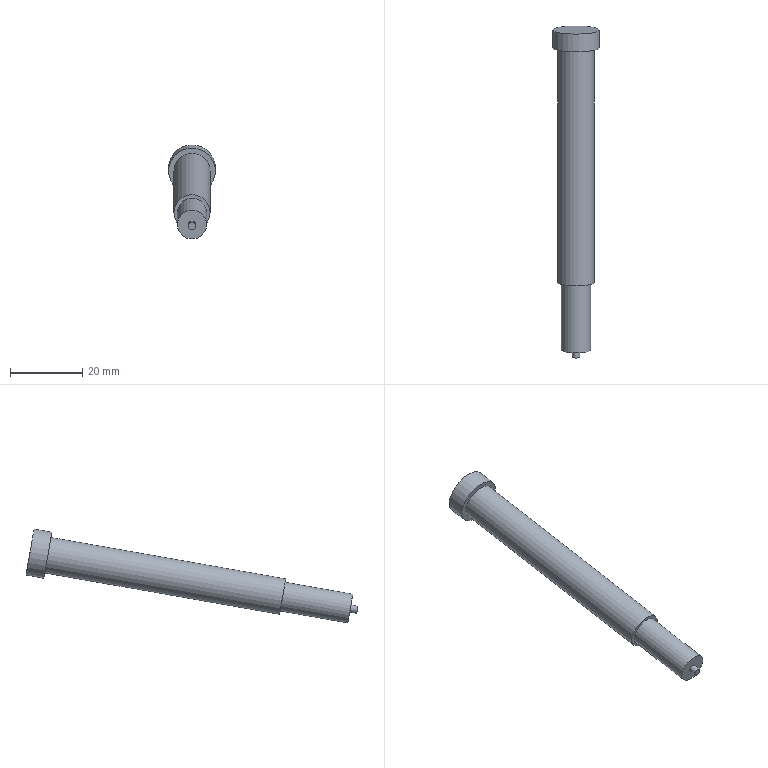Part | NX | features solid 2 | 1 solid | 9 faces | box 13 x 91.905 x 26.018 mm | volume 6833 mm3 | plane 5 | cylinder 4 | commonest cylinder face diameters 2 x1 8.1 x1 10 x1 13 x1
STEP:
#1=CARTESIAN_POINT('',(554.171,576.6,-0.1623));
#2=VERTEX_POINT('',#1);
#3=CARTESIAN_POINT('',(549.171,576.6,-0.1623));
#4=DIRECTION('',(0.,-0.9848,-0.1736));
#5=DIRECTION('',(1.,0.,0.));
#6=AXIS2_PLACEMENT_3D('',#3,#4,#5);
#7=CIRCLE('',#6,5.);
#8=EDGE_CURVE('',#2,#2,#7,.T.);
#9=ORIENTED_EDGE('',*,*,#8,.F.);
#10=EDGE_LOOP('',(#9));
#11=FACE_BOUND('',#10,.T.);
#12=CARTESIAN_POINT('',(554.171,641.597,11.298));
#13=VERTEX_POINT('',#12);
#14=CARTESIAN_POINT('',(549.171,641.597,11.298));
#15=DIRECTION('',(0.,-0.9848,-0.1736));
#16=DIRECTION('',(1.,0.,0.));
#17=AXIS2_PLACEMENT_3D('',#14,#15,#16);
#18=CIRCLE('',#17,5.);
#19=EDGE_CURVE('',#13,#13,#18,.T.);
#20=ORIENTED_EDGE('',*,*,#19,.T.);
#21=EDGE_LOOP('',(#20));
#22=FACE_BOUND('',#21,.T.);
#23=CARTESIAN_POINT('',(549.171,646.521,12.167));
#24=DIRECTION('',(0.,-0.9848,-0.1736));
#25=DIRECTION('',(-1.,0.,0.));
#26=AXIS2_PLACEMENT_3D('',#23,#24,#25);
#27=CYLINDRICAL_SURFACE('',#26,5.);
#28=ADVANCED_FACE('',(#11,#22),#27,.T.);
#29=CARTESIAN_POINT('',(553.221,576.6,-0.1623));
#30=VERTEX_POINT('',#29);
#31=CARTESIAN_POINT('',(549.171,576.6,-0.1623));
#32=DIRECTION('',(0.,-0.9848,-0.1736));
#33=DIRECTION('',(1.,0.,0.));
#34=AXIS2_PLACEMENT_3D('',#31,#32,#33);
#35=CIRCLE('',#34,4.05);
#36=EDGE_CURVE('',#30,#30,#35,.T.);
#37=ORIENTED_EDGE('',*,*,#36,.F.);
#38=EDGE_LOOP('',(#37));
#39=FACE_BOUND('',#38,.T.);
#40=ORIENTED_EDGE('',*,*,#8,.T.);
#41=EDGE_LOOP('',(#40));
#42=FACE_BOUND('',#41,.T.);
#43=CARTESIAN_POINT('',(549.171,576.6,-0.1623));
#44=DIRECTION('',(0.,0.9848,0.1736));
#45=DIRECTION('',(1.,0.,0.));
#46=AXIS2_PLACEMENT_3D('',#43,#44,#45);
#47=PLANE('',#46);
#48=ADVANCED_FACE('',(#39,#42),#47,.F.);
#49=CARTESIAN_POINT('',(555.671,641.597,11.298));
#50=VERTEX_POINT('',#49);
#51=CARTESIAN_POINT('',(549.171,641.597,11.298));
#52=DIRECTION('',(0.,-0.9848,-0.1736));
#53=DIRECTION('',(1.,0.,0.));
#54=AXIS2_PLACEMENT_3D('',#51,#52,#53);
#55=CIRCLE('',#54,6.5);
#56=EDGE_CURVE('',#50,#50,#55,.T.);
#57=ORIENTED_EDGE('',*,*,#56,.T.);
#58=EDGE_LOOP('',(#57));
#59=FACE_BOUND('',#58,.T.);
#60=ORIENTED_EDGE('',*,*,#19,.F.);
#61=EDGE_LOOP('',(#60));
#62=FACE_BOUND('',#61,.T.);
#63=CARTESIAN_POINT('',(549.171,641.597,11.298));
#64=DIRECTION('',(0.,0.9848,0.1736));
#65=DIRECTION('',(1.,0.,0.));
#66=AXIS2_PLACEMENT_3D('',#63,#64,#65);
#67=PLANE('',#66);
#68=ADVANCED_FACE('',(#59,#62),#67,.F.);
#69=ORIENTED_EDGE('',*,*,#56,.F.);
#70=EDGE_LOOP('',(#69));
#71=FACE_BOUND('',#70,.T.);
#72=CARTESIAN_POINT('',(555.671,646.521,12.167));
#73=VERTEX_POINT('',#72);
#74=CARTESIAN_POINT('',(549.171,646.521,12.167));
#75=DIRECTION('',(0.,-0.9848,-0.1736));
#76=DIRECTION('',(1.,0.,0.));
#77=AXIS2_PLACEMENT_3D('',#74,#75,#76);
#78=CIRCLE('',#77,6.5);
#79=EDGE_CURVE('',#73,#73,#78,.T.);
#80=ORIENTED_EDGE('',*,*,#79,.T.);
#81=EDGE_LOOP('',(#80));
#82=FACE_BOUND('',#81,.T.);
#83=CARTESIAN_POINT('',(549.171,641.597,11.298));
#84=DIRECTION('',(0.,0.9848,0.1736));
#85=DIRECTION('',(1.,0.,0.));
#86=AXIS2_PLACEMENT_3D('',#83,#84,#85);
#87=CYLINDRICAL_SURFACE('',#86,6.5);
#88=ADVANCED_FACE('',(#71,#82),#87,.T.);
#89=ORIENTED_EDGE('',*,*,#79,.F.);
#90=EDGE_LOOP('',(#89));
#91=FACE_BOUND('',#90,.T.);
#92=CARTESIAN_POINT('',(549.171,646.521,12.167));
#93=DIRECTION('',(0.,0.9848,0.1736));
#94=DIRECTION('',(1.,0.,0.));
#95=AXIS2_PLACEMENT_3D('',#92,#93,#94);
#96=PLANE('',#95);
#97=ADVANCED_FACE('',(#91),#96,.T.);
#98=CARTESIAN_POINT('',(553.221,557.888,-3.462));
#99=VERTEX_POINT('',#98);
#100=CARTESIAN_POINT('',(549.171,557.888,-3.462));
#101=DIRECTION('',(0.,-0.9848,-0.1736));
#102=DIRECTION('',(1.,0.,0.));
#103=AXIS2_PLACEMENT_3D('',#100,#101,#102);
#104=CIRCLE('',#103,4.05);
#105=EDGE_CURVE('',#99,#99,#104,.T.);
#106=ORIENTED_EDGE('',*,*,#105,.F.);
#107=EDGE_LOOP('',(#106));
#108=FACE_BOUND('',#107,.T.);
#109=ORIENTED_EDGE('',*,*,#36,.T.);
#110=EDGE_LOOP('',(#109));
#111=FACE_BOUND('',#110,.T.);
#112=CARTESIAN_POINT('',(549.171,557.888,-3.462));
#113=DIRECTION('',(0.,0.9848,0.1736));
#114=DIRECTION('',(1.,0.,0.));
#115=AXIS2_PLACEMENT_3D('',#112,#113,#114);
#116=CYLINDRICAL_SURFACE('',#115,4.05);
#117=ADVANCED_FACE('',(#108,#111),#116,.T.);
#118=CARTESIAN_POINT('',(550.171,557.888,-3.462));
#119=VERTEX_POINT('',#118);
#120=CARTESIAN_POINT('',(549.171,557.888,-3.462));
#121=DIRECTION('',(0.,-0.9848,-0.1736));
#122=DIRECTION('',(1.,0.,0.));
#123=AXIS2_PLACEMENT_3D('',#120,#121,#122);
#124=CIRCLE('',#123,1.);
#125=EDGE_CURVE('',#119,#119,#124,.T.);
#126=ORIENTED_EDGE('',*,*,#125,.F.);
#127=EDGE_LOOP('',(#126));
#128=FACE_BOUND('',#127,.T.);
#129=ORIENTED_EDGE('',*,*,#105,.T.);
#130=EDGE_LOOP('',(#129));
#131=FACE_BOUND('',#130,.T.);
#132=CARTESIAN_POINT('',(549.171,557.888,-3.462));
#133=DIRECTION('',(0.,0.9848,0.1736));
#134=DIRECTION('',(1.,0.,0.));
#135=AXIS2_PLACEMENT_3D('',#132,#133,#134);
#136=PLANE('',#135);
#137=ADVANCED_FACE('',(#128,#131),#136,.F.);
#138=CARTESIAN_POINT('',(550.171,555.919,-3.809));
#139=VERTEX_POINT('',#138);
#140=CARTESIAN_POINT('',(549.171,555.919,-3.809));
#141=DIRECTION('',(0.,-0.9848,-0.1736));
#142=DIRECTION('',(1.,0.,0.));
#143=AXIS2_PLACEMENT_3D('',#140,#141,#142);
#144=CIRCLE('',#143,1.);
#145=EDGE_CURVE('',#139,#139,#144,.T.);
#146=ORIENTED_EDGE('',*,*,#145,.F.);
#147=EDGE_LOOP('',(#146));
#148=FACE_BOUND('',#147,.T.);
#149=ORIENTED_EDGE('',*,*,#125,.T.);
#150=EDGE_LOOP('',(#149));
#151=FACE_BOUND('',#150,.T.);
#152=CARTESIAN_POINT('',(549.171,555.919,-3.809));
#153=DIRECTION('',(0.,0.9848,0.1736));
#154=DIRECTION('',(1.,0.,0.));
#155=AXIS2_PLACEMENT_3D('',#152,#153,#154);
#156=CYLINDRICAL_SURFACE('',#155,1.);
#157=ADVANCED_FACE('',(#148,#151),#156,.T.);
#158=ORIENTED_EDGE('',*,*,#145,.T.);
#159=EDGE_LOOP('',(#158));
#160=FACE_BOUND('',#159,.T.);
#161=CARTESIAN_POINT('',(549.171,555.919,-3.809));
#162=DIRECTION('',(0.,0.9848,0.1736));
#163=DIRECTION('',(1.,0.,0.));
#164=AXIS2_PLACEMENT_3D('',#161,#162,#163);
#165=PLANE('',#164);
#166=ADVANCED_FACE('',(#160),#165,.F.);
#167=CLOSED_SHELL('',(#28,#48,#68,#88,#97,#117,#137,#157,#166));
#168=MANIFOLD_SOLID_BREP('',#167);
#169=(LENGTH_UNIT()NAMED_UNIT(*)SI_UNIT(.MILLI.,.METRE.));
#170=UNCERTAINTY_MEASURE_WITH_UNIT(LENGTH_MEASURE(0.00001),#169,'','');
#171=(NAMED_UNIT(*)PLANE_ANGLE_UNIT()SI_UNIT($,.RADIAN.));
#172=(NAMED_UNIT(*)SI_UNIT($,.STERADIAN.)SOLID_ANGLE_UNIT());
#173=(GEOMETRIC_REPRESENTATION_CONTEXT(3)GLOBAL_UNCERTAINTY_ASSIGNED_CONTEXT((#170))GLOBAL_UNIT_ASSIGNED_CONTEXT((#169,#171,#172))REPRESENTATION_CONTEXT('',''));
#174=ADVANCED_BREP_SHAPE_REPRESENTATION('',(#168),#173);